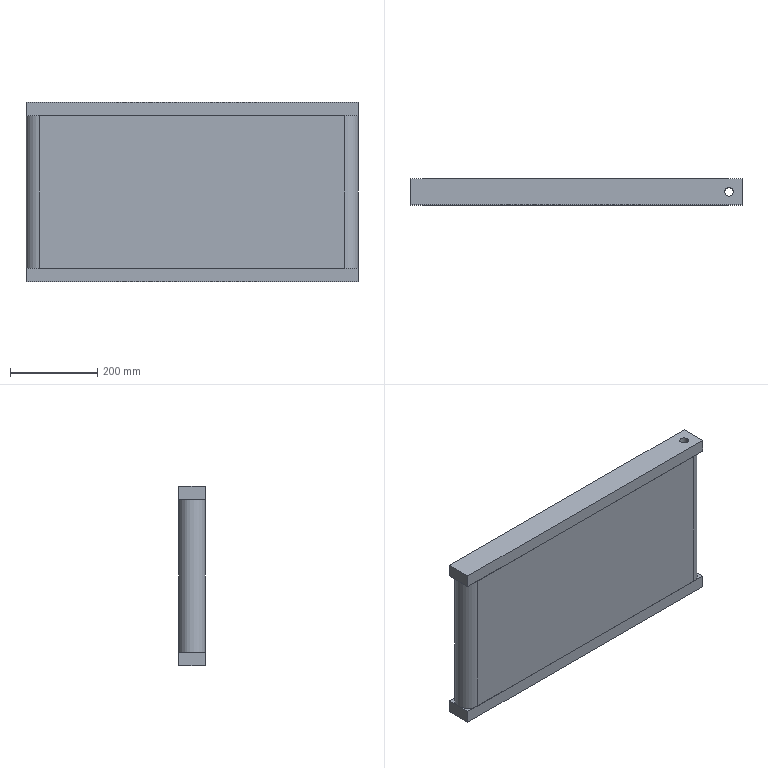Part | STEP file | 3 solids | 25 faces | box 760 x 60 x 410 mm | volume 18296796 mm3 | plane 16 | cylinder 9 | commonest cylinder face diameters 20 x6 60 x3